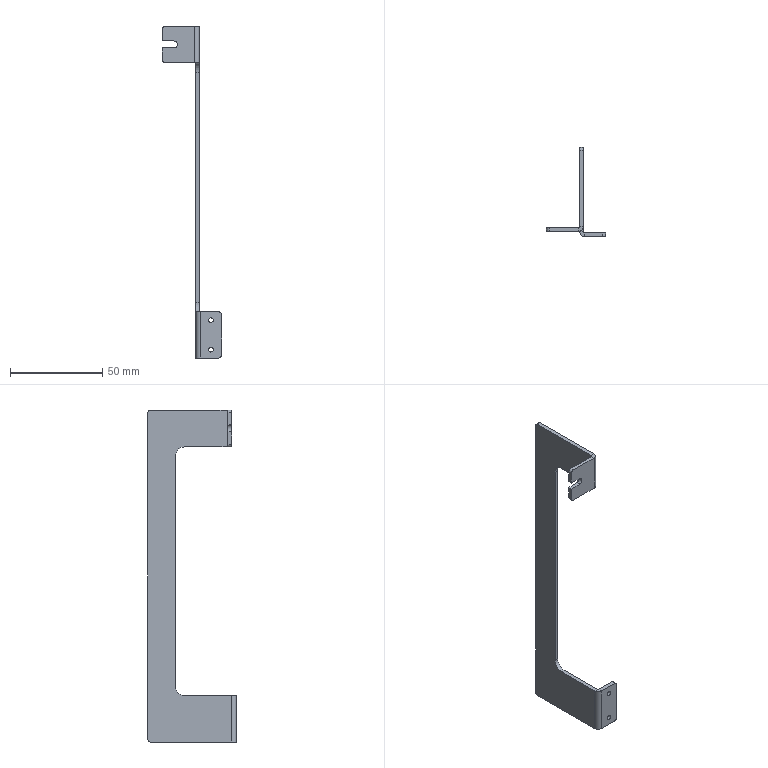Part | NX | features BREP 1 | 1 solid | 42 faces | box 32 x 48 x 180 mm | volume 9470 mm3 | plane 25 | cylinder 17 | commonest cylinder face diameters 3 x6 2.5 x4 1 x2 5 x2 10 x2 3.8 x1
STEP:
#1=CARTESIAN_POINT('',(-20.,-43.5,81.9));
#2=VERTEX_POINT('',#1);
#3=CARTESIAN_POINT('',(-20.,-45.5,81.9));
#4=VERTEX_POINT('',#3);
#5=CARTESIAN_POINT('',(-20.,-45.5,81.9));
#6=DIRECTION('',(0.,-1.,0.));
#7=VECTOR('',#6,1000.);
#8=LINE('',#5,#7);
#9=EDGE_CURVE('',#2,#4,#8,.T.);
#10=ORIENTED_EDGE('',*,*,#9,.F.);
#11=CARTESIAN_POINT('',(-13.9,-43.5,81.9));
#12=VERTEX_POINT('',#11);
#13=CARTESIAN_POINT('',(0.,-43.5,81.9));
#14=DIRECTION('',(1.,0.,0.));
#15=VECTOR('',#14,1000.);
#16=LINE('',#13,#15);
#17=EDGE_CURVE('',#2,#12,#16,.T.);
#18=ORIENTED_EDGE('',*,*,#17,.T.);
#19=CARTESIAN_POINT('',(-13.9,-45.5,81.9));
#20=VERTEX_POINT('',#19);
#21=CARTESIAN_POINT('',(-13.9,-43.5,81.9));
#22=DIRECTION('',(0.,-1.,0.));
#23=VECTOR('',#22,1000.);
#24=LINE('',#21,#23);
#25=EDGE_CURVE('',#12,#20,#24,.T.);
#26=ORIENTED_EDGE('',*,*,#25,.T.);
#27=CARTESIAN_POINT('',(0.,-45.5,81.9));
#28=DIRECTION('',(1.,0.,0.));
#29=VECTOR('',#28,1000.);
#30=LINE('',#27,#29);
#31=EDGE_CURVE('',#4,#20,#30,.T.);
#32=ORIENTED_EDGE('',*,*,#31,.F.);
#33=EDGE_LOOP('',(#10,#18,#26,#32));
#34=FACE_BOUND('',#33,.T.);
#35=CARTESIAN_POINT('',(-26.1,-43.5,81.9));
#36=DIRECTION('',(0.,0.,1.));
#37=DIRECTION('',(1.,0.,0.));
#38=AXIS2_PLACEMENT_3D('',#35,#36,#37);
#39=PLANE('',#38);
#40=ADVANCED_FACE('',(#34),#39,.F.);
#41=ORIENTED_EDGE('',*,*,#25,.F.);
#42=CARTESIAN_POINT('',(-13.9,-43.5,78.1));
#43=VERTEX_POINT('',#42);
#44=CARTESIAN_POINT('',(-13.9,-43.5,80.));
#45=DIRECTION('',(0.,1.,0.));
#46=DIRECTION('',(0.,0.,1.));
#47=AXIS2_PLACEMENT_3D('',#44,#45,#46);
#48=CIRCLE('',#47,1.9);
#49=EDGE_CURVE('',#12,#43,#48,.T.);
#50=ORIENTED_EDGE('',*,*,#49,.T.);
#51=CARTESIAN_POINT('',(-13.9,-45.5,78.1));
#52=VERTEX_POINT('',#51);
#53=CARTESIAN_POINT('',(-13.9,-43.5,78.1));
#54=DIRECTION('',(0.,1.,0.));
#55=VECTOR('',#54,1000.);
#56=LINE('',#53,#55);
#57=EDGE_CURVE('',#52,#43,#56,.T.);
#58=ORIENTED_EDGE('',*,*,#57,.F.);
#59=CARTESIAN_POINT('',(-13.9,-45.5,80.));
#60=DIRECTION('',(0.,1.,0.));
#61=DIRECTION('',(-1.,0.,0.));
#62=AXIS2_PLACEMENT_3D('',#59,#60,#61);
#63=CIRCLE('',#62,1.9);
#64=EDGE_CURVE('',#20,#52,#63,.T.);
#65=ORIENTED_EDGE('',*,*,#64,.F.);
#66=EDGE_LOOP('',(#41,#50,#58,#65));
#67=FACE_BOUND('',#66,.T.);
#68=CARTESIAN_POINT('',(-13.9,-43.5,80.));
#69=DIRECTION('',(0.,1.,0.));
#70=DIRECTION('',(0.,0.,1.));
#71=AXIS2_PLACEMENT_3D('',#68,#69,#70);
#72=CYLINDRICAL_SURFACE('',#71,1.9);
#73=ADVANCED_FACE('',(#67),#72,.F.);
#74=ORIENTED_EDGE('',*,*,#57,.T.);
#75=CARTESIAN_POINT('',(-20.,-43.5,78.1));
#76=VERTEX_POINT('',#75);
#77=CARTESIAN_POINT('',(0.,-43.5,78.1));
#78=DIRECTION('',(-1.,0.,0.));
#79=VECTOR('',#78,1000.);
#80=LINE('',#77,#79);
#81=EDGE_CURVE('',#43,#76,#80,.T.);
#82=ORIENTED_EDGE('',*,*,#81,.T.);
#83=CARTESIAN_POINT('',(-20.,-45.5,78.1));
#84=VERTEX_POINT('',#83);
#85=CARTESIAN_POINT('',(-20.,-45.5,78.1));
#86=DIRECTION('',(0.,1.,0.));
#87=VECTOR('',#86,1000.);
#88=LINE('',#85,#87);
#89=EDGE_CURVE('',#84,#76,#88,.T.);
#90=ORIENTED_EDGE('',*,*,#89,.F.);
#91=CARTESIAN_POINT('',(0.,-45.5,78.1));
#92=DIRECTION('',(-1.,0.,0.));
#93=VECTOR('',#92,1000.);
#94=LINE('',#91,#93);
#95=EDGE_CURVE('',#52,#84,#94,.T.);
#96=ORIENTED_EDGE('',*,*,#95,.F.);
#97=EDGE_LOOP('',(#74,#82,#90,#96));
#98=FACE_BOUND('',#97,.T.);
#99=CARTESIAN_POINT('',(-26.1,-43.5,78.1));
#100=DIRECTION('',(0.,0.,-1.));
#101=DIRECTION('',(-1.,0.,0.));
#102=AXIS2_PLACEMENT_3D('',#99,#100,#101);
#103=PLANE('',#102);
#104=ADVANCED_FACE('',(#98),#103,.F.);
#105=CARTESIAN_POINT('',(-2.,0.,-88.5));
#106=VERTEX_POINT('',#105);
#107=CARTESIAN_POINT('',(-2.,-1.5,-90.));
#108=VERTEX_POINT('',#107);
#109=CARTESIAN_POINT('',(-2.,-1.5,-88.5));
#110=DIRECTION('',(-1.,0.,0.));
#111=DIRECTION('',(0.,1.,0.));
#112=AXIS2_PLACEMENT_3D('',#109,#110,#111);
#113=CIRCLE('',#112,1.5);
#114=EDGE_CURVE('',#106,#108,#113,.T.);
#115=ORIENTED_EDGE('',*,*,#114,.F.);
#116=CARTESIAN_POINT('',(0.,0.,-88.5));
#117=VERTEX_POINT('',#116);
#118=CARTESIAN_POINT('',(-2.,0.,-88.5));
#119=DIRECTION('',(-1.,0.,0.));
#120=VECTOR('',#119,1000.);
#121=LINE('',#118,#120);
#122=EDGE_CURVE('',#117,#106,#121,.T.);
#123=ORIENTED_EDGE('',*,*,#122,.F.);
#124=CARTESIAN_POINT('',(0.,-1.5,-90.));
#125=VERTEX_POINT('',#124);
#126=CARTESIAN_POINT('',(0.,-1.5,-88.5));
#127=DIRECTION('',(1.,0.,0.));
#128=DIRECTION('',(0.,1.,0.));
#129=AXIS2_PLACEMENT_3D('',#126,#127,#128);
#130=CIRCLE('',#129,1.5);
#131=EDGE_CURVE('',#125,#117,#130,.T.);
#132=ORIENTED_EDGE('',*,*,#131,.F.);
#133=CARTESIAN_POINT('',(0.5,-1.5,-90.));
#134=DIRECTION('',(1.,0.,0.));
#135=VECTOR('',#134,1000.);
#136=LINE('',#133,#135);
#137=EDGE_CURVE('',#108,#125,#136,.T.);
#138=ORIENTED_EDGE('',*,*,#137,.F.);
#139=EDGE_LOOP('',(#115,#123,#132,#138));
#140=FACE_BOUND('',#139,.T.);
#141=CARTESIAN_POINT('',(0.5,-1.5,-88.5));
#142=DIRECTION('',(1.,0.,0.));
#143=DIRECTION('',(0.,1.,0.));
#144=AXIS2_PLACEMENT_3D('',#141,#142,#143);
#145=CYLINDRICAL_SURFACE('',#144,1.5);
#146=ADVANCED_FACE('',(#140),#145,.T.);
#147=CARTESIAN_POINT('',(-2.,-1.5,90.));
#148=VERTEX_POINT('',#147);
#149=CARTESIAN_POINT('',(-2.,0.,88.5));
#150=VERTEX_POINT('',#149);
#151=CARTESIAN_POINT('',(-2.,-1.5,88.5));
#152=DIRECTION('',(-1.,0.,0.));
#153=DIRECTION('',(0.,1.,0.));
#154=AXIS2_PLACEMENT_3D('',#151,#152,#153);
#155=CIRCLE('',#154,1.5);
#156=EDGE_CURVE('',#148,#150,#155,.T.);
#157=ORIENTED_EDGE('',*,*,#156,.F.);
#158=CARTESIAN_POINT('',(0.,-1.5,90.));
#159=VERTEX_POINT('',#158);
#160=CARTESIAN_POINT('',(-2.,-1.5,90.));
#161=DIRECTION('',(-1.,0.,0.));
#162=VECTOR('',#161,1000.);
#163=LINE('',#160,#162);
#164=EDGE_CURVE('',#159,#148,#163,.T.);
#165=ORIENTED_EDGE('',*,*,#164,.F.);
#166=CARTESIAN_POINT('',(0.,0.,88.5));
#167=VERTEX_POINT('',#166);
#168=CARTESIAN_POINT('',(0.,-1.5,88.5));
#169=DIRECTION('',(1.,0.,0.));
#170=DIRECTION('',(0.,1.,0.));
#171=AXIS2_PLACEMENT_3D('',#168,#169,#170);
#172=CIRCLE('',#171,1.5);
#173=EDGE_CURVE('',#167,#159,#172,.T.);
#174=ORIENTED_EDGE('',*,*,#173,.F.);
#175=CARTESIAN_POINT('',(0.,0.,88.5));
#176=DIRECTION('',(1.,0.,0.));
#177=VECTOR('',#176,1000.);
#178=LINE('',#175,#177);
#179=EDGE_CURVE('',#150,#167,#178,.T.);
#180=ORIENTED_EDGE('',*,*,#179,.F.);
#181=EDGE_LOOP('',(#157,#165,#174,#180));
#182=FACE_BOUND('',#181,.T.);
#183=CARTESIAN_POINT('',(-2.,-1.5,88.5));
#184=DIRECTION('',(-1.,0.,0.));
#185=DIRECTION('',(0.,-1.,0.));
#186=AXIS2_PLACEMENT_3D('',#183,#184,#185);
#187=CYLINDRICAL_SURFACE('',#186,1.5);
#188=ADVANCED_FACE('',(#182),#187,.T.);
#189=CARTESIAN_POINT('',(12.,-46.,-88.5));
#190=VERTEX_POINT('',#189);
#191=CARTESIAN_POINT('',(10.5,-46.,-90.));
#192=VERTEX_POINT('',#191);
#193=CARTESIAN_POINT('',(10.5,-46.,-88.5));
#194=DIRECTION('',(0.,1.,0.));
#195=DIRECTION('',(0.,0.,1.));
#196=AXIS2_PLACEMENT_3D('',#193,#194,#195);
#197=CIRCLE('',#196,1.5);
#198=EDGE_CURVE('',#190,#192,#197,.T.);
#199=ORIENTED_EDGE('',*,*,#198,.F.);
#200=CARTESIAN_POINT('',(12.,-48.,-88.5));
#201=VERTEX_POINT('',#200);
#202=CARTESIAN_POINT('',(12.,-46.,-88.5));
#203=DIRECTION('',(0.,1.,0.));
#204=VECTOR('',#203,1000.);
#205=LINE('',#202,#204);
#206=EDGE_CURVE('',#201,#190,#205,.T.);
#207=ORIENTED_EDGE('',*,*,#206,.F.);
#208=CARTESIAN_POINT('',(10.5,-48.,-90.));
#209=VERTEX_POINT('',#208);
#210=CARTESIAN_POINT('',(10.5,-48.,-88.5));
#211=DIRECTION('',(0.,-1.,0.));
#212=DIRECTION('',(0.,0.,1.));
#213=AXIS2_PLACEMENT_3D('',#210,#211,#212);
#214=CIRCLE('',#213,1.5);
#215=EDGE_CURVE('',#209,#201,#214,.T.);
#216=ORIENTED_EDGE('',*,*,#215,.F.);
#217=CARTESIAN_POINT('',(10.5,-45.5,-90.));
#218=DIRECTION('',(0.,-1.,0.));
#219=VECTOR('',#218,1000.);
#220=LINE('',#217,#219);
#221=EDGE_CURVE('',#192,#209,#220,.T.);
#222=ORIENTED_EDGE('',*,*,#221,.F.);
#223=EDGE_LOOP('',(#199,#207,#216,#222));
#224=FACE_BOUND('',#223,.T.);
#225=CARTESIAN_POINT('',(10.5,-45.5,-88.5));
#226=DIRECTION('',(0.,-1.,0.));
#227=DIRECTION('',(0.,0.,-1.));
#228=AXIS2_PLACEMENT_3D('',#225,#226,#227);
#229=CYLINDRICAL_SURFACE('',#228,1.5);
#230=ADVANCED_FACE('',(#224),#229,.T.);
#231=CARTESIAN_POINT('',(10.5,-46.,-65.));
#232=VERTEX_POINT('',#231);
#233=CARTESIAN_POINT('',(12.,-46.,-66.5));
#234=VERTEX_POINT('',#233);
#235=CARTESIAN_POINT('',(10.5,-46.,-66.5));
#236=DIRECTION('',(0.,1.,0.));
#237=DIRECTION('',(0.,0.,1.));
#238=AXIS2_PLACEMENT_3D('',#235,#236,#237);
#239=CIRCLE('',#238,1.5);
#240=EDGE_CURVE('',#232,#234,#239,.T.);
#241=ORIENTED_EDGE('',*,*,#240,.F.);
#242=CARTESIAN_POINT('',(10.5,-48.,-65.));
#243=VERTEX_POINT('',#242);
#244=CARTESIAN_POINT('',(10.5,-46.,-65.));
#245=DIRECTION('',(0.,1.,0.));
#246=VECTOR('',#245,1000.);
#247=LINE('',#244,#246);
#248=EDGE_CURVE('',#243,#232,#247,.T.);
#249=ORIENTED_EDGE('',*,*,#248,.F.);
#250=CARTESIAN_POINT('',(12.,-48.,-66.5));
#251=VERTEX_POINT('',#250);
#252=CARTESIAN_POINT('',(10.5,-48.,-66.5));
#253=DIRECTION('',(0.,-1.,0.));
#254=DIRECTION('',(0.,0.,1.));
#255=AXIS2_PLACEMENT_3D('',#252,#253,#254);
#256=CIRCLE('',#255,1.5);
#257=EDGE_CURVE('',#251,#243,#256,.T.);
#258=ORIENTED_EDGE('',*,*,#257,.F.);
#259=CARTESIAN_POINT('',(12.,-48.,-66.5));
#260=DIRECTION('',(0.,-1.,0.));
#261=VECTOR('',#260,1000.);
#262=LINE('',#259,#261);
#263=EDGE_CURVE('',#234,#251,#262,.T.);
#264=ORIENTED_EDGE('',*,*,#263,.F.);
#265=EDGE_LOOP('',(#241,#249,#258,#264));
#266=FACE_BOUND('',#265,.T.);
#267=CARTESIAN_POINT('',(10.5,-46.,-66.5));
#268=DIRECTION('',(0.,1.,0.));
#269=DIRECTION('',(0.,0.,1.));
#270=AXIS2_PLACEMENT_3D('',#267,#268,#269);
#271=CYLINDRICAL_SURFACE('',#270,1.5);
#272=ADVANCED_FACE('',(#266),#271,.T.);
#273=CARTESIAN_POINT('',(-18.5,-45.5,90.));
#274=VERTEX_POINT('',#273);
#275=CARTESIAN_POINT('',(-20.,-45.5,88.5));
#276=VERTEX_POINT('',#275);
#277=CARTESIAN_POINT('',(-18.5,-45.5,88.5));
#278=DIRECTION('',(0.,-1.,0.));
#279=DIRECTION('',(-1.,0.,0.));
#280=AXIS2_PLACEMENT_3D('',#277,#278,#279);
#281=CIRCLE('',#280,1.5);
#282=EDGE_CURVE('',#274,#276,#281,.T.);
#283=ORIENTED_EDGE('',*,*,#282,.F.);
#284=CARTESIAN_POINT('',(-18.5,-43.5,90.));
#285=VERTEX_POINT('',#284);
#286=CARTESIAN_POINT('',(-18.5,-45.5,90.));
#287=DIRECTION('',(0.,-1.,0.));
#288=VECTOR('',#287,1000.);
#289=LINE('',#286,#288);
#290=EDGE_CURVE('',#285,#274,#289,.T.);
#291=ORIENTED_EDGE('',*,*,#290,.F.);
#292=CARTESIAN_POINT('',(-20.,-43.5,88.5));
#293=VERTEX_POINT('',#292);
#294=CARTESIAN_POINT('',(-18.5,-43.5,88.5));
#295=DIRECTION('',(0.,1.,0.));
#296=DIRECTION('',(-1.,0.,0.));
#297=AXIS2_PLACEMENT_3D('',#294,#295,#296);
#298=CIRCLE('',#297,1.5);
#299=EDGE_CURVE('',#293,#285,#298,.T.);
#300=ORIENTED_EDGE('',*,*,#299,.F.);
#301=CARTESIAN_POINT('',(-20.,-45.5,88.5));
#302=DIRECTION('',(0.,1.,0.));
#303=VECTOR('',#302,1000.);
#304=LINE('',#301,#303);
#305=EDGE_CURVE('',#276,#293,#304,.T.);
#306=ORIENTED_EDGE('',*,*,#305,.F.);
#307=EDGE_LOOP('',(#283,#291,#300,#306));
#308=FACE_BOUND('',#307,.T.);
#309=CARTESIAN_POINT('',(-18.5,-45.5,88.5));
#310=DIRECTION('',(0.,1.,0.));
#311=DIRECTION('',(-1.,0.,0.));
#312=AXIS2_PLACEMENT_3D('',#309,#310,#311);
#313=CYLINDRICAL_SURFACE('',#312,1.5);
#314=ADVANCED_FACE('',(#308),#313,.T.);
#315=CARTESIAN_POINT('',(-20.,-45.5,71.5));
#316=VERTEX_POINT('',#315);
#317=CARTESIAN_POINT('',(-18.5,-45.5,70.));
#318=VERTEX_POINT('',#317);
#319=CARTESIAN_POINT('',(-18.5,-45.5,71.5));
#320=DIRECTION('',(0.,-1.,0.));
#321=DIRECTION('',(-1.,0.,0.));
#322=AXIS2_PLACEMENT_3D('',#319,#320,#321);
#323=CIRCLE('',#322,1.5);
#324=EDGE_CURVE('',#316,#318,#323,.T.);
#325=ORIENTED_EDGE('',*,*,#324,.F.);
#326=CARTESIAN_POINT('',(-20.,-43.5,71.5));
#327=VERTEX_POINT('',#326);
#328=CARTESIAN_POINT('',(-20.,-45.5,71.5));
#329=DIRECTION('',(0.,-1.,0.));
#330=VECTOR('',#329,1000.);
#331=LINE('',#328,#330);
#332=EDGE_CURVE('',#327,#316,#331,.T.);
#333=ORIENTED_EDGE('',*,*,#332,.F.);
#334=CARTESIAN_POINT('',(-18.5,-43.5,70.));
#335=VERTEX_POINT('',#334);
#336=CARTESIAN_POINT('',(-18.5,-43.5,71.5));
#337=DIRECTION('',(0.,1.,0.));
#338=DIRECTION('',(-1.,0.,0.));
#339=AXIS2_PLACEMENT_3D('',#336,#337,#338);
#340=CIRCLE('',#339,1.5);
#341=EDGE_CURVE('',#335,#327,#340,.T.);
#342=ORIENTED_EDGE('',*,*,#341,.F.);
#343=CARTESIAN_POINT('',(-18.5,-45.5,70.));
#344=DIRECTION('',(0.,1.,0.));
#345=VECTOR('',#344,1000.);
#346=LINE('',#343,#345);
#347=EDGE_CURVE('',#318,#335,#346,.T.);
#348=ORIENTED_EDGE('',*,*,#347,.F.);
#349=EDGE_LOOP('',(#325,#333,#342,#348));
#350=FACE_BOUND('',#349,.T.);
#351=CARTESIAN_POINT('',(-18.5,-45.5,71.5));
#352=DIRECTION('',(0.,1.,0.));
#353=DIRECTION('',(-1.,0.,0.));
#354=AXIS2_PLACEMENT_3D('',#351,#352,#353);
#355=CYLINDRICAL_SURFACE('',#354,1.5);
#356=ADVANCED_FACE('',(#350),#355,.T.);
#357=CARTESIAN_POINT('',(-20.,-45.5,0.));
#358=DIRECTION('',(0.,0.,-1.));
#359=VECTOR('',#358,1000.);
#360=LINE('',#357,#359);
#361=EDGE_CURVE('',#84,#316,#360,.T.);
#362=ORIENTED_EDGE('',*,*,#361,.F.);
#363=ORIENTED_EDGE('',*,*,#89,.T.);
#364=CARTESIAN_POINT('',(-20.,-43.5,70.));
#365=DIRECTION('',(0.,0.,-1.));
#366=VECTOR('',#365,1000.);
#367=LINE('',#364,#366);
#368=EDGE_CURVE('',#76,#327,#367,.T.);
#369=ORIENTED_EDGE('',*,*,#368,.T.);
#370=ORIENTED_EDGE('',*,*,#332,.T.);
#371=EDGE_LOOP('',(#362,#363,#369,#370));
#372=FACE_BOUND('',#371,.T.);
#373=CARTESIAN_POINT('',(-20.,-45.5,70.));
#374=DIRECTION('',(1.,0.,0.));
#375=DIRECTION('',(0.,1.,0.));
#376=AXIS2_PLACEMENT_3D('',#373,#374,#375);
#377=PLANE('',#376);
#378=ADVANCED_FACE('',(#372),#377,.F.);
#379=ORIENTED_EDGE('',*,*,#81,.F.);
#380=ORIENTED_EDGE('',*,*,#49,.F.);
#381=ORIENTED_EDGE('',*,*,#17,.F.);
#382=CARTESIAN_POINT('',(-20.,-43.5,70.));
#383=DIRECTION('',(0.,0.,-1.));
#384=VECTOR('',#383,1000.);
#385=LINE('',#382,#384);
#386=EDGE_CURVE('',#293,#2,#385,.T.);
#387=ORIENTED_EDGE('',*,*,#386,.F.);
#388=ORIENTED_EDGE('',*,*,#299,.T.);
#389=CARTESIAN_POINT('',(-2.5,-43.5,90.));
#390=VERTEX_POINT('',#389);
#391=CARTESIAN_POINT('',(-20.,-43.5,90.));
#392=DIRECTION('',(-1.,0.,0.));
#393=VECTOR('',#392,1000.);
#394=LINE('',#391,#393);
#395=EDGE_CURVE('',#390,#285,#394,.T.);
#396=ORIENTED_EDGE('',*,*,#395,.F.);
#397=CARTESIAN_POINT('',(-2.5,-43.5,70.));
#398=VERTEX_POINT('',#397);
#399=CARTESIAN_POINT('',(-2.5,-43.5,70.));
#400=DIRECTION('',(0.,0.,1.));
#401=VECTOR('',#400,1000.);
#402=LINE('',#399,#401);
#403=EDGE_CURVE('',#398,#390,#402,.T.);
#404=ORIENTED_EDGE('',*,*,#403,.F.);
#405=CARTESIAN_POINT('',(-2.,-43.5,70.));
#406=DIRECTION('',(1.,0.,0.));
#407=VECTOR('',#406,1000.);
#408=LINE('',#405,#407);
#409=EDGE_CURVE('',#335,#398,#408,.T.);
#410=ORIENTED_EDGE('',*,*,#409,.F.);
#411=ORIENTED_EDGE('',*,*,#341,.T.);
#412=ORIENTED_EDGE('',*,*,#368,.F.);
#413=EDGE_LOOP('',(#379,#380,#381,#387,#388,#396,#404,#410,#411,#412));
#414=FACE_BOUND('',#413,.T.);
#415=CARTESIAN_POINT('',(0.,-43.5,0.));
#416=DIRECTION('',(0.,1.,0.));
#417=DIRECTION('',(-1.,0.,0.));
#418=AXIS2_PLACEMENT_3D('',#415,#416,#417);
#419=PLANE('',#418);
#420=ADVANCED_FACE('',(#414),#419,.T.);
#421=ORIENTED_EDGE('',*,*,#64,.T.);
#422=ORIENTED_EDGE('',*,*,#95,.T.);
#423=ORIENTED_EDGE('',*,*,#361,.T.);
#424=ORIENTED_EDGE('',*,*,#324,.T.);
#425=CARTESIAN_POINT('',(-2.5,-45.5,70.));
#426=VERTEX_POINT('',#425);
#427=CARTESIAN_POINT('',(0.,-45.5,70.));
#428=DIRECTION('',(1.,0.,0.));
#429=VECTOR('',#428,1000.);
#430=LINE('',#427,#429);
#431=EDGE_CURVE('',#318,#426,#430,.T.);
#432=ORIENTED_EDGE('',*,*,#431,.T.);
#433=CARTESIAN_POINT('',(-2.5,-45.5,90.));
#434=VERTEX_POINT('',#433);
#435=CARTESIAN_POINT('',(-2.5,-45.5,70.));
#436=DIRECTION('',(0.,0.,-1.));
#437=VECTOR('',#436,1000.);
#438=LINE('',#435,#437);
#439=EDGE_CURVE('',#434,#426,#438,.T.);
#440=ORIENTED_EDGE('',*,*,#439,.F.);
#441=CARTESIAN_POINT('',(0.,-45.5,90.));
#442=DIRECTION('',(-1.,0.,0.));
#443=VECTOR('',#442,1000.);
#444=LINE('',#441,#443);
#445=EDGE_CURVE('',#434,#274,#444,.T.);
#446=ORIENTED_EDGE('',*,*,#445,.T.);
#447=ORIENTED_EDGE('',*,*,#282,.T.);
#448=CARTESIAN_POINT('',(-20.,-45.5,0.));
#449=DIRECTION('',(0.,0.,-1.));
#450=VECTOR('',#449,1000.);
#451=LINE('',#448,#450);
#452=EDGE_CURVE('',#276,#4,#451,.T.);
#453=ORIENTED_EDGE('',*,*,#452,.T.);
#454=ORIENTED_EDGE('',*,*,#31,.T.);
#455=EDGE_LOOP('',(#421,#422,#423,#424,#432,#440,#446,#447,#453,#454));
#456=FACE_BOUND('',#455,.T.);
#457=CARTESIAN_POINT('',(0.,-45.5,0.));
#458=DIRECTION('',(0.,1.,0.));
#459=DIRECTION('',(-1.,0.,0.));
#460=AXIS2_PLACEMENT_3D('',#457,#458,#459);
#461=PLANE('',#460);
#462=ADVANCED_FACE('',(#456),#461,.F.);
#463=ORIENTED_EDGE('',*,*,#395,.T.);
#464=ORIENTED_EDGE('',*,*,#290,.T.);
#465=ORIENTED_EDGE('',*,*,#445,.F.);
#466=CARTESIAN_POINT('',(-2.5,-43.5,90.));
#467=DIRECTION('',(0.,-1.,0.));
#468=VECTOR('',#467,1000.);
#469=LINE('',#466,#468);
#470=EDGE_CURVE('',#390,#434,#469,.T.);
#471=ORIENTED_EDGE('',*,*,#470,.F.);
#472=EDGE_LOOP('',(#463,#464,#465,#471));
#473=FACE_BOUND('',#472,.T.);
#474=CARTESIAN_POINT('',(-20.,-45.5,90.));
#475=DIRECTION('',(0.,0.,-1.));
#476=DIRECTION('',(-1.,0.,0.));
#477=AXIS2_PLACEMENT_3D('',#474,#475,#476);
#478=PLANE('',#477);
#479=ADVANCED_FACE('',(#473),#478,.F.);
#480=ORIENTED_EDGE('',*,*,#431,.F.);
#481=ORIENTED_EDGE('',*,*,#347,.T.);
#482=ORIENTED_EDGE('',*,*,#409,.T.);
#483=CARTESIAN_POINT('',(-2.5,-45.5,70.));
#484=DIRECTION('',(0.,-1.,0.));
#485=VECTOR('',#484,1000.);
#486=LINE('',#483,#485);
#487=EDGE_CURVE('',#398,#426,#486,.T.);
#488=ORIENTED_EDGE('',*,*,#487,.T.);
#489=EDGE_LOOP('',(#480,#481,#482,#488));
#490=FACE_BOUND('',#489,.T.);
#491=CARTESIAN_POINT('',(-2.,-45.5,70.));
#492=DIRECTION('',(0.,0.,1.));
#493=DIRECTION('',(1.,0.,0.));
#494=AXIS2_PLACEMENT_3D('',#491,#492,#493);
#495=PLANE('',#494);
#496=ADVANCED_FACE('',(#490),#495,.F.);
#497=CARTESIAN_POINT('',(-2.,-43.,90.));
#498=VERTEX_POINT('',#497);
#499=CARTESIAN_POINT('',(-2.,-43.,70.));
#500=VERTEX_POINT('',#499);
#501=CARTESIAN_POINT('',(-2.,-43.,90.));
#502=DIRECTION('',(0.,0.,-1.));
#503=VECTOR('',#502,1000.);
#504=LINE('',#501,#503);
#505=EDGE_CURVE('',#498,#500,#504,.T.);
#506=ORIENTED_EDGE('',*,*,#505,.T.);
#507=CARTESIAN_POINT('',(-2.5,-43.,70.));
#508=DIRECTION('',(0.,0.,-1.));
#509=DIRECTION('',(1.,0.,0.));
#510=AXIS2_PLACEMENT_3D('',#507,#508,#509);
#511=CIRCLE('',#510,0.5);
#512=EDGE_CURVE('',#500,#398,#511,.T.);
#513=ORIENTED_EDGE('',*,*,#512,.T.);
#514=ORIENTED_EDGE('',*,*,#403,.T.);
#515=CARTESIAN_POINT('',(-2.5,-43.,90.));
#516=DIRECTION('',(0.,0.,1.));
#517=DIRECTION('',(1.,0.,0.));
#518=AXIS2_PLACEMENT_3D('',#515,#516,#517);
#519=CIRCLE('',#518,0.5);
#520=EDGE_CURVE('',#390,#498,#519,.T.);
#521=ORIENTED_EDGE('',*,*,#520,.T.);
#522=EDGE_LOOP('',(#506,#513,#514,#521));
#523=FACE_BOUND('',#522,.T.);
#524=CARTESIAN_POINT('',(-2.5,-43.,90.));
#525=DIRECTION('',(0.,0.,1.));
#526=DIRECTION('',(0.,-1.,0.));
#527=AXIS2_PLACEMENT_3D('',#524,#525,#526);
#528=CYLINDRICAL_SURFACE('',#527,0.5);
#529=ADVANCED_FACE('',(#523),#528,.F.);
#530=CARTESIAN_POINT('',(0.,-43.,90.));
#531=VERTEX_POINT('',#530);
#532=CARTESIAN_POINT('',(0.,-43.,70.));
#533=VERTEX_POINT('',#532);
#534=CARTESIAN_POINT('',(0.,-43.,90.));
#535=DIRECTION('',(0.,0.,-1.));
#536=VECTOR('',#535,1000.);
#537=LINE('',#534,#536);
#538=EDGE_CURVE('',#531,#533,#537,.T.);
#539=ORIENTED_EDGE('',*,*,#538,.F.);
#540=CARTESIAN_POINT('',(-2.5,-43.,90.));
#541=DIRECTION('',(0.,0.,1.));
#542=DIRECTION('',(1.,0.,0.));
#543=AXIS2_PLACEMENT_3D('',#540,#541,#542);
#544=CIRCLE('',#543,2.5);
#545=EDGE_CURVE('',#434,#531,#544,.T.);
#546=ORIENTED_EDGE('',*,*,#545,.F.);
#547=ORIENTED_EDGE('',*,*,#439,.T.);
#548=CARTESIAN_POINT('',(-2.5,-43.,70.));
#549=DIRECTION('',(0.,0.,-1.));
#550=DIRECTION('',(1.,0.,0.));
#551=AXIS2_PLACEMENT_3D('',#548,#549,#550);
#552=CIRCLE('',#551,2.5);
#553=EDGE_CURVE('',#533,#426,#552,.T.);
#554=ORIENTED_EDGE('',*,*,#553,.F.);
#555=EDGE_LOOP('',(#539,#546,#547,#554));
#556=FACE_BOUND('',#555,.T.);
#557=CARTESIAN_POINT('',(-2.5,-43.,90.));
#558=DIRECTION('',(0.,0.,1.));
#559=DIRECTION('',(0.,-1.,0.));
#560=AXIS2_PLACEMENT_3D('',#557,#558,#559);
#561=CYLINDRICAL_SURFACE('',#560,2.5);
#562=ADVANCED_FACE('',(#556),#561,.T.);
#563=ORIENTED_EDGE('',*,*,#520,.F.);
#564=ORIENTED_EDGE('',*,*,#470,.T.);
#565=ORIENTED_EDGE('',*,*,#545,.T.);
#566=CARTESIAN_POINT('',(-2.,-43.,90.));
#567=DIRECTION('',(1.,0.,0.));
#568=VECTOR('',#567,1000.);
#569=LINE('',#566,#568);
#570=EDGE_CURVE('',#498,#531,#569,.T.);
#571=ORIENTED_EDGE('',*,*,#570,.F.);
#572=EDGE_LOOP('',(#563,#564,#565,#571));
#573=FACE_BOUND('',#572,.T.);
#574=CARTESIAN_POINT('',(-2.5,-43.,90.));
#575=DIRECTION('',(0.,0.,-1.));
#576=DIRECTION('',(-1.,0.,0.));
#577=AXIS2_PLACEMENT_3D('',#574,#575,#576);
#578=PLANE('',#577);
#579=ADVANCED_FACE('',(#573),#578,.F.);
#580=ORIENTED_EDGE('',*,*,#487,.F.);
#581=ORIENTED_EDGE('',*,*,#512,.F.);
#582=CARTESIAN_POINT('',(-2.,-43.,70.));
#583=DIRECTION('',(1.,0.,0.));
#584=VECTOR('',#583,1000.);
#585=LINE('',#582,#584);
#586=EDGE_CURVE('',#500,#533,#585,.T.);
#587=ORIENTED_EDGE('',*,*,#586,.T.);
#588=ORIENTED_EDGE('',*,*,#553,.T.);
#589=EDGE_LOOP('',(#580,#581,#587,#588));
#590=FACE_BOUND('',#589,.T.);
#591=CARTESIAN_POINT('',(-2.5,-43.,70.));
#592=DIRECTION('',(0.,0.,-1.));
#593=DIRECTION('',(-1.,0.,0.));
#594=AXIS2_PLACEMENT_3D('',#591,#592,#593);
#595=PLANE('',#594);
#596=ADVANCED_FACE('',(#590),#595,.T.);
#597=CARTESIAN_POINT('',(0.,-15.,-60.));
#598=VERTEX_POINT('',#597);
#599=CARTESIAN_POINT('',(0.,-20.,-65.));
#600=VERTEX_POINT('',#599);
#601=CARTESIAN_POINT('',(0.,-20.,-60.));
#602=DIRECTION('',(-1.,0.,0.));
#603=DIRECTION('',(0.,1.,0.));
#604=AXIS2_PLACEMENT_3D('',#601,#602,#603);
#605=CIRCLE('',#604,5.);
#606=EDGE_CURVE('',#598,#600,#605,.T.);
#607=ORIENTED_EDGE('',*,*,#606,.F.);
#608=CARTESIAN_POINT('',(-2.,-15.,-60.));
#609=VERTEX_POINT('',#608);
#610=CARTESIAN_POINT('',(0.,-15.,-60.));
#611=DIRECTION('',(1.,0.,0.));
#612=VECTOR('',#611,1000.);
#613=LINE('',#610,#612);
#614=EDGE_CURVE('',#609,#598,#613,.T.);
#615=ORIENTED_EDGE('',*,*,#614,.F.);
#616=CARTESIAN_POINT('',(-2.,-20.,-65.));
#617=VERTEX_POINT('',#616);
#618=CARTESIAN_POINT('',(-2.,-20.,-60.));
#619=DIRECTION('',(1.,0.,0.));
#620=DIRECTION('',(0.,1.,0.));
#621=AXIS2_PLACEMENT_3D('',#618,#619,#620);
#622=CIRCLE('',#621,5.);
#623=EDGE_CURVE('',#617,#609,#622,.T.);
#624=ORIENTED_EDGE('',*,*,#623,.F.);
#625=CARTESIAN_POINT('',(-2.,-20.,-65.));
#626=DIRECTION('',(-1.,0.,0.));
#627=VECTOR('',#626,1000.);
#628=LINE('',#625,#627);
#629=EDGE_CURVE('',#600,#617,#628,.T.);
#630=ORIENTED_EDGE('',*,*,#629,.F.);
#631=EDGE_LOOP('',(#607,#615,#624,#630));
#632=FACE_BOUND('',#631,.T.);
#633=CARTESIAN_POINT('',(12.,-20.,-60.));
#634=DIRECTION('',(1.,0.,0.));
#635=DIRECTION('',(0.,1.,0.));
#636=AXIS2_PLACEMENT_3D('',#633,#634,#635);
#637=CYLINDRICAL_SURFACE('',#636,5.);
#638=ADVANCED_FACE('',(#632),#637,.F.);
#639=CARTESIAN_POINT('',(0.,-20.,70.));
#640=VERTEX_POINT('',#639);
#641=CARTESIAN_POINT('',(0.,-15.,65.));
#642=VERTEX_POINT('',#641);
#643=CARTESIAN_POINT('',(0.,-20.,65.));
#644=DIRECTION('',(-1.,0.,0.));
#645=DIRECTION('',(0.,1.,0.));
#646=AXIS2_PLACEMENT_3D('',#643,#644,#645);
#647=CIRCLE('',#646,5.);
#648=EDGE_CURVE('',#640,#642,#647,.T.);
#649=ORIENTED_EDGE('',*,*,#648,.F.);
#650=CARTESIAN_POINT('',(-2.,-20.,70.));
#651=VERTEX_POINT('',#650);
#652=CARTESIAN_POINT('',(0.,-20.,70.));
#653=DIRECTION('',(1.,0.,0.));
#654=VECTOR('',#653,1000.);
#655=LINE('',#652,#654);
#656=EDGE_CURVE('',#651,#640,#655,.T.);
#657=ORIENTED_EDGE('',*,*,#656,.F.);
#658=CARTESIAN_POINT('',(-2.,-15.,65.));
#659=VERTEX_POINT('',#658);
#660=CARTESIAN_POINT('',(-2.,-20.,65.));
#661=DIRECTION('',(1.,0.,0.));
#662=DIRECTION('',(0.,1.,0.));
#663=AXIS2_PLACEMENT_3D('',#660,#661,#662);
#664=CIRCLE('',#663,5.);
#665=EDGE_CURVE('',#659,#651,#664,.T.);
#666=ORIENTED_EDGE('',*,*,#665,.F.);
#667=CARTESIAN_POINT('',(-2.,-15.,65.));
#668=DIRECTION('',(-1.,0.,0.));
#669=VECTOR('',#668,1000.);
#670=LINE('',#667,#669);
#671=EDGE_CURVE('',#642,#659,#670,.T.);
#672=ORIENTED_EDGE('',*,*,#671,.F.);
#673=EDGE_LOOP('',(#649,#657,#666,#672));
#674=FACE_BOUND('',#673,.T.);
#675=CARTESIAN_POINT('',(12.,-20.,65.));
#676=DIRECTION('',(1.,0.,0.));
#677=DIRECTION('',(0.,1.,0.));
#678=AXIS2_PLACEMENT_3D('',#675,#676,#677);
#679=CYLINDRICAL_SURFACE('',#678,5.);
#680=ADVANCED_FACE('',(#674),#679,.F.);
#681=CARTESIAN_POINT('',(6.25,-46.,-68.25));
#682=VERTEX_POINT('',#681);
#683=CARTESIAN_POINT('',(6.25,-48.,-68.25));
#684=VERTEX_POINT('',#683);
#685=CARTESIAN_POINT('',(6.25,-48.,-68.25));
#686=DIRECTION('',(0.,-1.,0.));
#687=VECTOR('',#686,1000.);
#688=LINE('',#685,#687);
#689=EDGE_CURVE('',#682,#684,#688,.T.);
#690=ORIENTED_EDGE('',*,*,#689,.F.);
#691=CARTESIAN_POINT('',(6.25,-46.,-70.75));
#692=VERTEX_POINT('',#691);
#693=CARTESIAN_POINT('',(6.25,-46.,-69.5));
#694=DIRECTION('',(0.,1.,0.));
#695=DIRECTION('',(0.,0.,1.));
#696=AXIS2_PLACEMENT_3D('',#693,#694,#695);
#697=CIRCLE('',#696,1.25);
#698=EDGE_CURVE('',#682,#692,#697,.T.);
#699=ORIENTED_EDGE('',*,*,#698,.T.);
#700=CARTESIAN_POINT('',(6.25,-48.,-70.75));
#701=VERTEX_POINT('',#700);
#702=CARTESIAN_POINT('',(6.25,-48.,-70.75));
#703=DIRECTION('',(0.,-1.,0.));
#704=VECTOR('',#703,1000.);
#705=LINE('',#702,#704);
#706=EDGE_CURVE('',#692,#701,#705,.T.);
#707=ORIENTED_EDGE('',*,*,#706,.T.);
#708=CARTESIAN_POINT('',(6.25,-48.,-69.5));
#709=DIRECTION('',(0.,-1.,0.));
#710=DIRECTION('',(0.,0.,-1.));
#711=AXIS2_PLACEMENT_3D('',#708,#709,#710);
#712=CIRCLE('',#711,1.25);
#713=EDGE_CURVE('',#701,#684,#712,.T.);
#714=ORIENTED_EDGE('',*,*,#713,.T.);
#715=EDGE_LOOP('',(#690,#699,#707,#714));
#716=FACE_BOUND('',#715,.T.);
#717=CARTESIAN_POINT('',(6.25,-48.,-69.5));
#718=DIRECTION('',(0.,-1.,0.));
#719=DIRECTION('',(0.,0.,-1.));
#720=AXIS2_PLACEMENT_3D('',#717,#718,#719);
#721=CYLINDRICAL_SURFACE('',#720,1.25);
#722=ADVANCED_FACE('',(#716),#721,.F.);
#723=CARTESIAN_POINT('',(6.25,-46.,-84.25));
#724=VERTEX_POINT('',#723);
#725=CARTESIAN_POINT('',(6.25,-48.,-84.25));
#726=VERTEX_POINT('',#725);
#727=CARTESIAN_POINT('',(6.25,-48.,-84.25));
#728=DIRECTION('',(0.,-1.,0.));
#729=VECTOR('',#728,1000.);
#730=LINE('',#727,#729);
#731=EDGE_CURVE('',#724,#726,#730,.T.);
#732=ORIENTED_EDGE('',*,*,#731,.F.);
#733=CARTESIAN_POINT('',(6.25,-46.,-86.75));
#734=VERTEX_POINT('',#733);
#735=CARTESIAN_POINT('',(6.25,-46.,-85.5));
#736=DIRECTION('',(0.,1.,0.));
#737=DIRECTION('',(0.,0.,1.));
#738=AXIS2_PLACEMENT_3D('',#735,#736,#737);
#739=CIRCLE('',#738,1.25);
#740=EDGE_CURVE('',#724,#734,#739,.T.);
#741=ORIENTED_EDGE('',*,*,#740,.T.);
#742=CARTESIAN_POINT('',(6.25,-48.,-86.75));
#743=VERTEX_POINT('',#742);
#744=CARTESIAN_POINT('',(6.25,-48.,-86.75));
#745=DIRECTION('',(0.,-1.,0.));
#746=VECTOR('',#745,1000.);
#747=LINE('',#744,#746);
#748=EDGE_CURVE('',#734,#743,#747,.T.);
#749=ORIENTED_EDGE('',*,*,#748,.T.);
#750=CARTESIAN_POINT('',(6.25,-48.,-85.5));
#751=DIRECTION('',(0.,-1.,0.));
#752=DIRECTION('',(0.,0.,-1.));
#753=AXIS2_PLACEMENT_3D('',#750,#751,#752);
#754=CIRCLE('',#753,1.25);
#755=EDGE_CURVE('',#743,#726,#754,.T.);
#756=ORIENTED_EDGE('',*,*,#755,.T.);
#757=EDGE_LOOP('',(#732,#741,#749,#756));
#758=FACE_BOUND('',#757,.T.);
#759=CARTESIAN_POINT('',(6.25,-48.,-85.5));
#760=DIRECTION('',(0.,-1.,0.));
#761=DIRECTION('',(0.,0.,-1.));
#762=AXIS2_PLACEMENT_3D('',#759,#760,#761);
#763=CYLINDRICAL_SURFACE('',#762,1.25);
#764=ADVANCED_FACE('',(#758),#763,.F.);
#765=CARTESIAN_POINT('',(0.,-15.,90.));
#766=DIRECTION('',(0.,0.,1.));
#767=VECTOR('',#766,1000.);
#768=LINE('',#765,#767);
#769=EDGE_CURVE('',#598,#642,#768,.T.);
#770=ORIENTED_EDGE('',*,*,#769,.T.);
#771=ORIENTED_EDGE('',*,*,#671,.T.);
#772=CARTESIAN_POINT('',(-2.,-15.,-65.));
#773=DIRECTION('',(0.,0.,-1.));
#774=VECTOR('',#773,1000.);
#775=LINE('',#772,#774);
#776=EDGE_CURVE('',#659,#609,#775,.T.);
#777=ORIENTED_EDGE('',*,*,#776,.T.);
#778=ORIENTED_EDGE('',*,*,#614,.T.);
#779=EDGE_LOOP('',(#770,#771,#777,#778));
#780=FACE_BOUND('',#779,.T.);
#781=CARTESIAN_POINT('',(12.,-15.,-65.));
#782=DIRECTION('',(0.,1.,0.));
#783=DIRECTION('',(-1.,0.,0.));
#784=AXIS2_PLACEMENT_3D('',#781,#782,#783);
#785=PLANE('',#784);
#786=ADVANCED_FACE('',(#780),#785,.F.);
#787=CARTESIAN_POINT('',(-2.,-45.5,-65.));
#788=VERTEX_POINT('',#787);
#789=CARTESIAN_POINT('',(0.,-45.5,-65.));
#790=VERTEX_POINT('',#789);
#791=CARTESIAN_POINT('',(-2.,-45.5,-65.));
#792=DIRECTION('',(1.,0.,0.));
#793=VECTOR('',#792,1000.);
#794=LINE('',#791,#793);
#795=EDGE_CURVE('',#788,#790,#794,.T.);
#796=ORIENTED_EDGE('',*,*,#795,.F.);
#797=CARTESIAN_POINT('',(0.5,-48.,-65.));
#798=VERTEX_POINT('',#797);
#799=CARTESIAN_POINT('',(0.5,-45.5,-65.));
#800=DIRECTION('',(0.,0.,-1.));
#801=DIRECTION('',(0.,1.,0.));
#802=AXIS2_PLACEMENT_3D('',#799,#800,#801);
#803=CIRCLE('',#802,2.5);
#804=EDGE_CURVE('',#798,#788,#803,.T.);
#805=ORIENTED_EDGE('',*,*,#804,.F.);
#806=CARTESIAN_POINT('',(0.5,-46.,-65.));
#807=VERTEX_POINT('',#806);
#808=CARTESIAN_POINT('',(0.5,-46.,-65.));
#809=DIRECTION('',(0.,-1.,0.));
#810=VECTOR('',#809,1000.);
#811=LINE('',#808,#810);
#812=EDGE_CURVE('',#807,#798,#811,.T.);
#813=ORIENTED_EDGE('',*,*,#812,.F.);
#814=CARTESIAN_POINT('',(0.5,-45.5,-65.));
#815=DIRECTION('',(0.,0.,-1.));
#816=DIRECTION('',(0.,1.,0.));
#817=AXIS2_PLACEMENT_3D('',#814,#815,#816);
#818=CIRCLE('',#817,0.5);
#819=EDGE_CURVE('',#807,#790,#818,.T.);
#820=ORIENTED_EDGE('',*,*,#819,.T.);
#821=EDGE_LOOP('',(#796,#805,#813,#820));
#822=FACE_BOUND('',#821,.T.);
#823=CARTESIAN_POINT('',(12.,-48.,-65.));
#824=DIRECTION('',(0.,0.,-1.));
#825=DIRECTION('',(0.,1.,0.));
#826=AXIS2_PLACEMENT_3D('',#823,#824,#825);
#827=PLANE('',#826);
#828=ADVANCED_FACE('',(#822),#827,.F.);
#829=CARTESIAN_POINT('',(0.5,-46.,-90.));
#830=VERTEX_POINT('',#829);
#831=CARTESIAN_POINT('',(0.,-46.,-90.));
#832=DIRECTION('',(1.,0.,0.));
#833=VECTOR('',#832,1000.);
#834=LINE('',#831,#833);
#835=EDGE_CURVE('',#830,#192,#834,.T.);
#836=ORIENTED_EDGE('',*,*,#835,.T.);
#837=ORIENTED_EDGE('',*,*,#221,.T.);
#838=CARTESIAN_POINT('',(0.5,-48.,-90.));
#839=VERTEX_POINT('',#838);
#840=CARTESIAN_POINT('',(0.,-48.,-90.));
#841=DIRECTION('',(1.,0.,0.));
#842=VECTOR('',#841,1000.);
#843=LINE('',#840,#842);
#844=EDGE_CURVE('',#839,#209,#843,.T.);
#845=ORIENTED_EDGE('',*,*,#844,.F.);
#846=CARTESIAN_POINT('',(0.5,-48.,-90.));
#847=DIRECTION('',(0.,1.,0.));
#848=VECTOR('',#847,1000.);
#849=LINE('',#846,#848);
#850=EDGE_CURVE('',#839,#830,#849,.T.);
#851=ORIENTED_EDGE('',*,*,#850,.T.);
#852=EDGE_LOOP('',(#836,#837,#845,#851));
#853=FACE_BOUND('',#852,.T.);
#854=CARTESIAN_POINT('',(0.5,-45.5,-90.));
#855=DIRECTION('',(0.,0.,-1.));
#856=DIRECTION('',(-1.,0.,0.));
#857=AXIS2_PLACEMENT_3D('',#854,#855,#856);
#858=PLANE('',#857);
#859=ADVANCED_FACE('',(#853),#858,.T.);
#860=CARTESIAN_POINT('',(-2.,0.,90.));
#861=DIRECTION('',(0.,0.,-1.));
#862=VECTOR('',#861,1000.);
#863=LINE('',#860,#862);
#864=EDGE_CURVE('',#150,#106,#863,.T.);
#865=ORIENTED_EDGE('',*,*,#864,.F.);
#866=ORIENTED_EDGE('',*,*,#179,.T.);
#867=CARTESIAN_POINT('',(0.,0.,90.));
#868=DIRECTION('',(0.,0.,-1.));
#869=VECTOR('',#868,1000.);
#870=LINE('',#867,#869);
#871=EDGE_CURVE('',#167,#117,#870,.T.);
#872=ORIENTED_EDGE('',*,*,#871,.T.);
#873=ORIENTED_EDGE('',*,*,#122,.T.);
#874=EDGE_LOOP('',(#865,#866,#872,#873));
#875=FACE_BOUND('',#874,.T.);
#876=CARTESIAN_POINT('',(-2.,0.,90.));
#877=DIRECTION('',(0.,1.,0.));
#878=DIRECTION('',(-1.,0.,0.));
#879=AXIS2_PLACEMENT_3D('',#876,#877,#878);
#880=PLANE('',#879);
#881=ADVANCED_FACE('',(#875),#880,.T.);
#882=CARTESIAN_POINT('',(-2.,-45.5,-90.));
#883=VERTEX_POINT('',#882);
#884=CARTESIAN_POINT('',(-2.,0.,-90.));
#885=DIRECTION('',(0.,-1.,0.));
#886=VECTOR('',#885,1000.);
#887=LINE('',#884,#886);
#888=EDGE_CURVE('',#108,#883,#887,.T.);
#889=ORIENTED_EDGE('',*,*,#888,.F.);
#890=ORIENTED_EDGE('',*,*,#137,.T.);
#891=CARTESIAN_POINT('',(0.,-45.5,-90.));
#892=VERTEX_POINT('',#891);
#893=CARTESIAN_POINT('',(0.,0.,-90.));
#894=DIRECTION('',(0.,-1.,0.));
#895=VECTOR('',#894,1000.);
#896=LINE('',#893,#895);
#897=EDGE_CURVE('',#125,#892,#896,.T.);
#898=ORIENTED_EDGE('',*,*,#897,.T.);
#899=CARTESIAN_POINT('',(0.,-45.5,-90.));
#900=DIRECTION('',(-1.,0.,0.));
#901=VECTOR('',#900,1000.);
#902=LINE('',#899,#901);
#903=EDGE_CURVE('',#892,#883,#902,.T.);
#904=ORIENTED_EDGE('',*,*,#903,.T.);
#905=EDGE_LOOP('',(#889,#890,#898,#904));
#906=FACE_BOUND('',#905,.T.);
#907=CARTESIAN_POINT('',(0.5,-48.,-90.));
#908=DIRECTION('',(0.,0.,-1.));
#909=DIRECTION('',(-1.,0.,0.));
#910=AXIS2_PLACEMENT_3D('',#907,#908,#909);
#911=PLANE('',#910);
#912=ADVANCED_FACE('',(#906),#911,.T.);
#913=ORIENTED_EDGE('',*,*,#903,.F.);
#914=CARTESIAN_POINT('',(0.5,-45.5,-90.));
#915=DIRECTION('',(0.,0.,1.));
#916=DIRECTION('',(-1.,0.,0.));
#917=AXIS2_PLACEMENT_3D('',#914,#915,#916);
#918=CIRCLE('',#917,0.5);
#919=EDGE_CURVE('',#892,#830,#918,.T.);
#920=ORIENTED_EDGE('',*,*,#919,.T.);
#921=ORIENTED_EDGE('',*,*,#850,.F.);
#922=CARTESIAN_POINT('',(0.5,-45.5,-90.));
#923=DIRECTION('',(0.,0.,1.));
#924=DIRECTION('',(1.,0.,0.));
#925=AXIS2_PLACEMENT_3D('',#922,#923,#924);
#926=CIRCLE('',#925,2.5);
#927=EDGE_CURVE('',#883,#839,#926,.T.);
#928=ORIENTED_EDGE('',*,*,#927,.F.);
#929=EDGE_LOOP('',(#913,#920,#921,#928));
#930=FACE_BOUND('',#929,.T.);
#931=CARTESIAN_POINT('',(0.,-45.5,-90.));
#932=DIRECTION('',(0.,0.,-1.));
#933=DIRECTION('',(-1.,0.,0.));
#934=AXIS2_PLACEMENT_3D('',#931,#932,#933);
#935=PLANE('',#934);
#936=ADVANCED_FACE('',(#930),#935,.T.);
#937=CARTESIAN_POINT('',(0.5,-48.,90.));
#938=DIRECTION('',(0.,0.,-1.));
#939=VECTOR('',#938,1000.);
#940=LINE('',#937,#939);
#941=EDGE_CURVE('',#798,#839,#940,.T.);
#942=ORIENTED_EDGE('',*,*,#941,.F.);
#943=ORIENTED_EDGE('',*,*,#804,.T.);
#944=CARTESIAN_POINT('',(-2.,-45.5,90.));
#945=DIRECTION('',(0.,0.,-1.));
#946=VECTOR('',#945,1000.);
#947=LINE('',#944,#946);
#948=EDGE_CURVE('',#788,#883,#947,.T.);
#949=ORIENTED_EDGE('',*,*,#948,.T.);
#950=ORIENTED_EDGE('',*,*,#927,.T.);
#951=EDGE_LOOP('',(#942,#943,#949,#950));
#952=FACE_BOUND('',#951,.T.);
#953=CARTESIAN_POINT('',(0.5,-45.5,90.));
#954=DIRECTION('',(0.,0.,-1.));
#955=DIRECTION('',(-1.,0.,0.));
#956=AXIS2_PLACEMENT_3D('',#953,#954,#955);
#957=CYLINDRICAL_SURFACE('',#956,2.5);
#958=ADVANCED_FACE('',(#952),#957,.T.);
#959=ORIENTED_EDGE('',*,*,#819,.F.);
#960=CARTESIAN_POINT('',(0.5,-46.,90.));
#961=DIRECTION('',(0.,0.,-1.));
#962=VECTOR('',#961,1000.);
#963=LINE('',#960,#962);
#964=EDGE_CURVE('',#807,#830,#963,.T.);
#965=ORIENTED_EDGE('',*,*,#964,.T.);
#966=ORIENTED_EDGE('',*,*,#919,.F.);
#967=CARTESIAN_POINT('',(0.,-45.5,90.));
#968=DIRECTION('',(0.,0.,-1.));
#969=VECTOR('',#968,1000.);
#970=LINE('',#967,#969);
#971=EDGE_CURVE('',#790,#892,#970,.T.);
#972=ORIENTED_EDGE('',*,*,#971,.F.);
#973=EDGE_LOOP('',(#959,#965,#966,#972));
#974=FACE_BOUND('',#973,.T.);
#975=CARTESIAN_POINT('',(0.5,-45.5,90.));
#976=DIRECTION('',(0.,0.,-1.));
#977=DIRECTION('',(-1.,0.,0.));
#978=AXIS2_PLACEMENT_3D('',#975,#976,#977);
#979=CYLINDRICAL_SURFACE('',#978,0.5);
#980=ADVANCED_FACE('',(#974),#979,.F.);
#981=CARTESIAN_POINT('',(0.,-46.,-65.));
#982=DIRECTION('',(-1.,0.,0.));
#983=VECTOR('',#982,1000.);
#984=LINE('',#981,#983);
#985=EDGE_CURVE('',#232,#807,#984,.T.);
#986=ORIENTED_EDGE('',*,*,#985,.F.);
#987=ORIENTED_EDGE('',*,*,#240,.T.);
#988=CARTESIAN_POINT('',(12.,-46.,90.));
#989=DIRECTION('',(0.,0.,-1.));
#990=VECTOR('',#989,1000.);
#991=LINE('',#988,#990);
#992=EDGE_CURVE('',#234,#190,#991,.T.);
#993=ORIENTED_EDGE('',*,*,#992,.T.);
#994=ORIENTED_EDGE('',*,*,#198,.T.);
#995=ORIENTED_EDGE('',*,*,#835,.F.);
#996=ORIENTED_EDGE('',*,*,#964,.F.);
#997=EDGE_LOOP('',(#986,#987,#993,#994,#995,#996));
#998=FACE_BOUND('',#997,.T.);
#999=CARTESIAN_POINT('',(6.25,-46.,-85.5));
#1000=DIRECTION('',(0.,1.,0.));
#1001=DIRECTION('',(0.,0.,1.));
#1002=AXIS2_PLACEMENT_3D('',#999,#1000,#1001);
#1003=CIRCLE('',#1002,1.25);
#1004=EDGE_CURVE('',#734,#724,#1003,.T.);
#1005=ORIENTED_EDGE('',*,*,#1004,.F.);
#1006=ORIENTED_EDGE('',*,*,#740,.F.);
#1007=EDGE_LOOP('',(#1005,#1006));
#1008=FACE_BOUND('',#1007,.T.);
#1009=CARTESIAN_POINT('',(6.25,-46.,-69.5));
#1010=DIRECTION('',(0.,1.,0.));
#1011=DIRECTION('',(0.,0.,1.));
#1012=AXIS2_PLACEMENT_3D('',#1009,#1010,#1011);
#1013=CIRCLE('',#1012,1.25);
#1014=EDGE_CURVE('',#692,#682,#1013,.T.);
#1015=ORIENTED_EDGE('',*,*,#1014,.F.);
#1016=ORIENTED_EDGE('',*,*,#698,.F.);
#1017=EDGE_LOOP('',(#1015,#1016));
#1018=FACE_BOUND('',#1017,.T.);
#1019=CARTESIAN_POINT('',(0.,-46.,90.));
#1020=DIRECTION('',(0.,1.,0.));
#1021=DIRECTION('',(0.,0.,1.));
#1022=AXIS2_PLACEMENT_3D('',#1019,#1020,#1021);
#1023=PLANE('',#1022);
#1024=ADVANCED_FACE('',(#998,#1008,#1018),#1023,.T.);
#1025=ORIENTED_EDGE('',*,*,#992,.F.);
#1026=ORIENTED_EDGE('',*,*,#263,.T.);
#1027=CARTESIAN_POINT('',(12.,-48.,90.));
#1028=DIRECTION('',(0.,0.,-1.));
#1029=VECTOR('',#1028,1000.);
#1030=LINE('',#1027,#1029);
#1031=EDGE_CURVE('',#251,#201,#1030,.T.);
#1032=ORIENTED_EDGE('',*,*,#1031,.T.);
#1033=ORIENTED_EDGE('',*,*,#206,.T.);
#1034=EDGE_LOOP('',(#1025,#1026,#1032,#1033));
#1035=FACE_BOUND('',#1034,.T.);
#1036=CARTESIAN_POINT('',(12.,-46.,90.));
#1037=DIRECTION('',(1.,0.,0.));
#1038=DIRECTION('',(0.,0.,-1.));
#1039=AXIS2_PLACEMENT_3D('',#1036,#1037,#1038);
#1040=PLANE('',#1039);
#1041=ADVANCED_FACE('',(#1035),#1040,.T.);
#1042=ORIENTED_EDGE('',*,*,#1031,.F.);
#1043=ORIENTED_EDGE('',*,*,#257,.T.);
#1044=CARTESIAN_POINT('',(12.,-48.,-65.));
#1045=DIRECTION('',(-1.,0.,0.));
#1046=VECTOR('',#1045,1000.);
#1047=LINE('',#1044,#1046);
#1048=EDGE_CURVE('',#243,#798,#1047,.T.);
#1049=ORIENTED_EDGE('',*,*,#1048,.T.);
#1050=ORIENTED_EDGE('',*,*,#941,.T.);
#1051=ORIENTED_EDGE('',*,*,#844,.T.);
#1052=ORIENTED_EDGE('',*,*,#215,.T.);
#1053=EDGE_LOOP('',(#1042,#1043,#1049,#1050,#1051,#1052));
#1054=FACE_BOUND('',#1053,.T.);
#1055=ORIENTED_EDGE('',*,*,#755,.F.);
#1056=CARTESIAN_POINT('',(6.25,-48.,-85.5));
#1057=DIRECTION('',(0.,-1.,0.));
#1058=DIRECTION('',(0.,0.,-1.));
#1059=AXIS2_PLACEMENT_3D('',#1056,#1057,#1058);
#1060=CIRCLE('',#1059,1.25);
#1061=EDGE_CURVE('',#726,#743,#1060,.T.);
#1062=ORIENTED_EDGE('',*,*,#1061,.F.);
#1063=EDGE_LOOP('',(#1055,#1062));
#1064=FACE_BOUND('',#1063,.T.);
#1065=ORIENTED_EDGE('',*,*,#713,.F.);
#1066=CARTESIAN_POINT('',(6.25,-48.,-69.5));
#1067=DIRECTION('',(0.,-1.,0.));
#1068=DIRECTION('',(0.,0.,-1.));
#1069=AXIS2_PLACEMENT_3D('',#1066,#1067,#1068);
#1070=CIRCLE('',#1069,1.25);
#1071=EDGE_CURVE('',#684,#701,#1070,.T.);
#1072=ORIENTED_EDGE('',*,*,#1071,.F.);
#1073=EDGE_LOOP('',(#1065,#1072));
#1074=FACE_BOUND('',#1073,.T.);
#1075=CARTESIAN_POINT('',(0.,-48.,90.));
#1076=DIRECTION('',(0.,1.,0.));
#1077=DIRECTION('',(0.,0.,1.));
#1078=AXIS2_PLACEMENT_3D('',#1075,#1076,#1077);
#1079=PLANE('',#1078);
#1080=ADVANCED_FACE('',(#1054,#1064,#1074),#1079,.F.);
#1081=ORIENTED_EDGE('',*,*,#1048,.F.);
#1082=ORIENTED_EDGE('',*,*,#248,.T.);
#1083=ORIENTED_EDGE('',*,*,#985,.T.);
#1084=ORIENTED_EDGE('',*,*,#812,.T.);
#1085=EDGE_LOOP('',(#1081,#1082,#1083,#1084));
#1086=FACE_BOUND('',#1085,.T.);
#1087=CARTESIAN_POINT('',(12.,-48.,-65.));
#1088=DIRECTION('',(0.,0.,-1.));
#1089=DIRECTION('',(0.,1.,0.));
#1090=AXIS2_PLACEMENT_3D('',#1087,#1088,#1089);
#1091=PLANE('',#1090);
#1092=ADVANCED_FACE('',(#1086),#1091,.F.);
#1093=CARTESIAN_POINT('',(0.,0.,-65.));
#1094=DIRECTION('',(0.,1.,0.));
#1095=VECTOR('',#1094,1000.);
#1096=LINE('',#1093,#1095);
#1097=EDGE_CURVE('',#790,#600,#1096,.T.);
#1098=ORIENTED_EDGE('',*,*,#1097,.T.);
#1099=ORIENTED_EDGE('',*,*,#629,.T.);
#1100=CARTESIAN_POINT('',(-2.,-48.,-65.));
#1101=DIRECTION('',(0.,-1.,0.));
#1102=VECTOR('',#1101,1000.);
#1103=LINE('',#1100,#1102);
#1104=EDGE_CURVE('',#617,#788,#1103,.T.);
#1105=ORIENTED_EDGE('',*,*,#1104,.T.);
#1106=ORIENTED_EDGE('',*,*,#795,.T.);
#1107=EDGE_LOOP('',(#1098,#1099,#1105,#1106));
#1108=FACE_BOUND('',#1107,.T.);
#1109=CARTESIAN_POINT('',(12.,-48.,-65.));
#1110=DIRECTION('',(0.,0.,-1.));
#1111=DIRECTION('',(0.,1.,0.));
#1112=AXIS2_PLACEMENT_3D('',#1109,#1110,#1111);
#1113=PLANE('',#1112);
#1114=ADVANCED_FACE('',(#1108),#1113,.F.);
#1115=CARTESIAN_POINT('',(0.,0.,90.));
#1116=DIRECTION('',(0.,-1.,0.));
#1117=VECTOR('',#1116,1000.);
#1118=LINE('',#1115,#1117);
#1119=EDGE_CURVE('',#159,#531,#1118,.T.);
#1120=ORIENTED_EDGE('',*,*,#1119,.F.);
#1121=ORIENTED_EDGE('',*,*,#164,.T.);
#1122=CARTESIAN_POINT('',(-2.,0.,90.));
#1123=DIRECTION('',(0.,-1.,0.));
#1124=VECTOR('',#1123,1000.);
#1125=LINE('',#1122,#1124);
#1126=EDGE_CURVE('',#148,#498,#1125,.T.);
#1127=ORIENTED_EDGE('',*,*,#1126,.T.);
#1128=ORIENTED_EDGE('',*,*,#570,.T.);
#1129=EDGE_LOOP('',(#1120,#1121,#1127,#1128));
#1130=FACE_BOUND('',#1129,.T.);
#1131=CARTESIAN_POINT('',(0.5,-45.5,90.));
#1132=DIRECTION('',(0.,0.,-1.));
#1133=DIRECTION('',(-1.,0.,0.));
#1134=AXIS2_PLACEMENT_3D('',#1131,#1132,#1133);
#1135=PLANE('',#1134);
#1136=ADVANCED_FACE('',(#1130),#1135,.F.);
#1137=ORIENTED_EDGE('',*,*,#1126,.F.);
#1138=ORIENTED_EDGE('',*,*,#156,.T.);
#1139=ORIENTED_EDGE('',*,*,#864,.T.);
#1140=ORIENTED_EDGE('',*,*,#114,.T.);
#1141=ORIENTED_EDGE('',*,*,#888,.T.);
#1142=ORIENTED_EDGE('',*,*,#948,.F.);
#1143=ORIENTED_EDGE('',*,*,#1104,.F.);
#1144=ORIENTED_EDGE('',*,*,#623,.T.);
#1145=ORIENTED_EDGE('',*,*,#776,.F.);
#1146=ORIENTED_EDGE('',*,*,#665,.T.);
#1147=CARTESIAN_POINT('',(-2.,-48.,70.));
#1148=DIRECTION('',(0.,1.,0.));
#1149=VECTOR('',#1148,1000.);
#1150=LINE('',#1147,#1149);
#1151=EDGE_CURVE('',#500,#651,#1150,.T.);
#1152=ORIENTED_EDGE('',*,*,#1151,.F.);
#1153=ORIENTED_EDGE('',*,*,#505,.F.);
#1154=EDGE_LOOP('',(#1137,#1138,#1139,#1140,#1141,#1142,#1143,#1144,#1145,#1146,#1152,#1153));
#1155=FACE_BOUND('',#1154,.T.);
#1156=CARTESIAN_POINT('',(-2.,0.,90.));
#1157=DIRECTION('',(1.,0.,0.));
#1158=DIRECTION('',(0.,1.,0.));
#1159=AXIS2_PLACEMENT_3D('',#1156,#1157,#1158);
#1160=PLANE('',#1159);
#1161=ADVANCED_FACE('',(#1155),#1160,.F.);
#1162=ORIENTED_EDGE('',*,*,#871,.F.);
#1163=ORIENTED_EDGE('',*,*,#173,.T.);
#1164=ORIENTED_EDGE('',*,*,#1119,.T.);
#1165=ORIENTED_EDGE('',*,*,#538,.T.);
#1166=CARTESIAN_POINT('',(0.,0.,70.));
#1167=DIRECTION('',(0.,-1.,0.));
#1168=VECTOR('',#1167,1000.);
#1169=LINE('',#1166,#1168);
#1170=EDGE_CURVE('',#640,#533,#1169,.T.);
#1171=ORIENTED_EDGE('',*,*,#1170,.F.);
#1172=ORIENTED_EDGE('',*,*,#648,.T.);
#1173=ORIENTED_EDGE('',*,*,#769,.F.);
#1174=ORIENTED_EDGE('',*,*,#606,.T.);
#1175=ORIENTED_EDGE('',*,*,#1097,.F.);
#1176=ORIENTED_EDGE('',*,*,#971,.T.);
#1177=ORIENTED_EDGE('',*,*,#897,.F.);
#1178=ORIENTED_EDGE('',*,*,#131,.T.);
#1179=EDGE_LOOP('',(#1162,#1163,#1164,#1165,#1171,#1172,#1173,#1174,#1175,#1176,#1177,#1178));
#1180=FACE_BOUND('',#1179,.T.);
#1181=CARTESIAN_POINT('',(0.,0.,90.));
#1182=DIRECTION('',(1.,0.,0.));
#1183=DIRECTION('',(0.,1.,0.));
#1184=AXIS2_PLACEMENT_3D('',#1181,#1182,#1183);
#1185=PLANE('',#1184);
#1186=ADVANCED_FACE('',(#1180),#1185,.T.);
#1187=ORIENTED_EDGE('',*,*,#586,.F.);
#1188=ORIENTED_EDGE('',*,*,#1151,.T.);
#1189=ORIENTED_EDGE('',*,*,#656,.T.);
#1190=ORIENTED_EDGE('',*,*,#1170,.T.);
#1191=EDGE_LOOP('',(#1187,#1188,#1189,#1190));
#1192=FACE_BOUND('',#1191,.T.);
#1193=CARTESIAN_POINT('',(12.,-48.,70.));
#1194=DIRECTION('',(0.,0.,1.));
#1195=DIRECTION('',(0.,-1.,0.));
#1196=AXIS2_PLACEMENT_3D('',#1193,#1194,#1195);
#1197=PLANE('',#1196);
#1198=ADVANCED_FACE('',(#1192),#1197,.F.);
#1199=ORIENTED_EDGE('',*,*,#386,.T.);
#1200=ORIENTED_EDGE('',*,*,#9,.T.);
#1201=ORIENTED_EDGE('',*,*,#452,.F.);
#1202=ORIENTED_EDGE('',*,*,#305,.T.);
#1203=EDGE_LOOP('',(#1199,#1200,#1201,#1202));
#1204=FACE_BOUND('',#1203,.T.);
#1205=CARTESIAN_POINT('',(-20.,-45.5,70.));
#1206=DIRECTION('',(1.,0.,0.));
#1207=DIRECTION('',(0.,1.,0.));
#1208=AXIS2_PLACEMENT_3D('',#1205,#1206,#1207);
#1209=PLANE('',#1208);
#1210=ADVANCED_FACE('',(#1204),#1209,.F.);
#1211=ORIENTED_EDGE('',*,*,#1004,.T.);
#1212=ORIENTED_EDGE('',*,*,#731,.T.);
#1213=ORIENTED_EDGE('',*,*,#1061,.T.);
#1214=ORIENTED_EDGE('',*,*,#748,.F.);
#1215=EDGE_LOOP('',(#1211,#1212,#1213,#1214));
#1216=FACE_BOUND('',#1215,.T.);
#1217=CARTESIAN_POINT('',(6.25,-48.,-85.5));
#1218=DIRECTION('',(0.,-1.,0.));
#1219=DIRECTION('',(0.,0.,-1.));
#1220=AXIS2_PLACEMENT_3D('',#1217,#1218,#1219);
#1221=CYLINDRICAL_SURFACE('',#1220,1.25);
#1222=ADVANCED_FACE('',(#1216),#1221,.F.);
#1223=ORIENTED_EDGE('',*,*,#1014,.T.);
#1224=ORIENTED_EDGE('',*,*,#689,.T.);
#1225=ORIENTED_EDGE('',*,*,#1071,.T.);
#1226=ORIENTED_EDGE('',*,*,#706,.F.);
#1227=EDGE_LOOP('',(#1223,#1224,#1225,#1226));
#1228=FACE_BOUND('',#1227,.T.);
#1229=CARTESIAN_POINT('',(6.25,-48.,-69.5));
#1230=DIRECTION('',(0.,-1.,0.));
#1231=DIRECTION('',(0.,0.,-1.));
#1232=AXIS2_PLACEMENT_3D('',#1229,#1230,#1231);
#1233=CYLINDRICAL_SURFACE('',#1232,1.25);
#1234=ADVANCED_FACE('',(#1228),#1233,.F.);
#1235=CLOSED_SHELL('',(#40,#73,#104,#146,#188,#230,#272,#314,#356,#378,#420,#462,#479,#496,#529,#562,#579,#596,#638,#680,#722,#764,#786,#828,#859,#881,#912,#936,#958,#980,#1024,#1041,#1080,#1092,#1114,#1136,#1161,#1186,#1198,#1210,#1222,#1234));
#1236=MANIFOLD_SOLID_BREP('',#1235);
#1237=(LENGTH_UNIT()NAMED_UNIT(*)SI_UNIT(.MILLI.,.METRE.));
#1238=UNCERTAINTY_MEASURE_WITH_UNIT(LENGTH_MEASURE(0.00001),#1237,'','');
#1239=(NAMED_UNIT(*)PLANE_ANGLE_UNIT()SI_UNIT($,.RADIAN.));
#1240=(NAMED_UNIT(*)SI_UNIT($,.STERADIAN.)SOLID_ANGLE_UNIT());
#1241=(GEOMETRIC_REPRESENTATION_CONTEXT(3)GLOBAL_UNCERTAINTY_ASSIGNED_CONTEXT((#1238))GLOBAL_UNIT_ASSIGNED_CONTEXT((#1237,#1239,#1240))REPRESENTATION_CONTEXT('',''));
#1242=ADVANCED_BREP_SHAPE_REPRESENTATION('',(#1236),#1241);